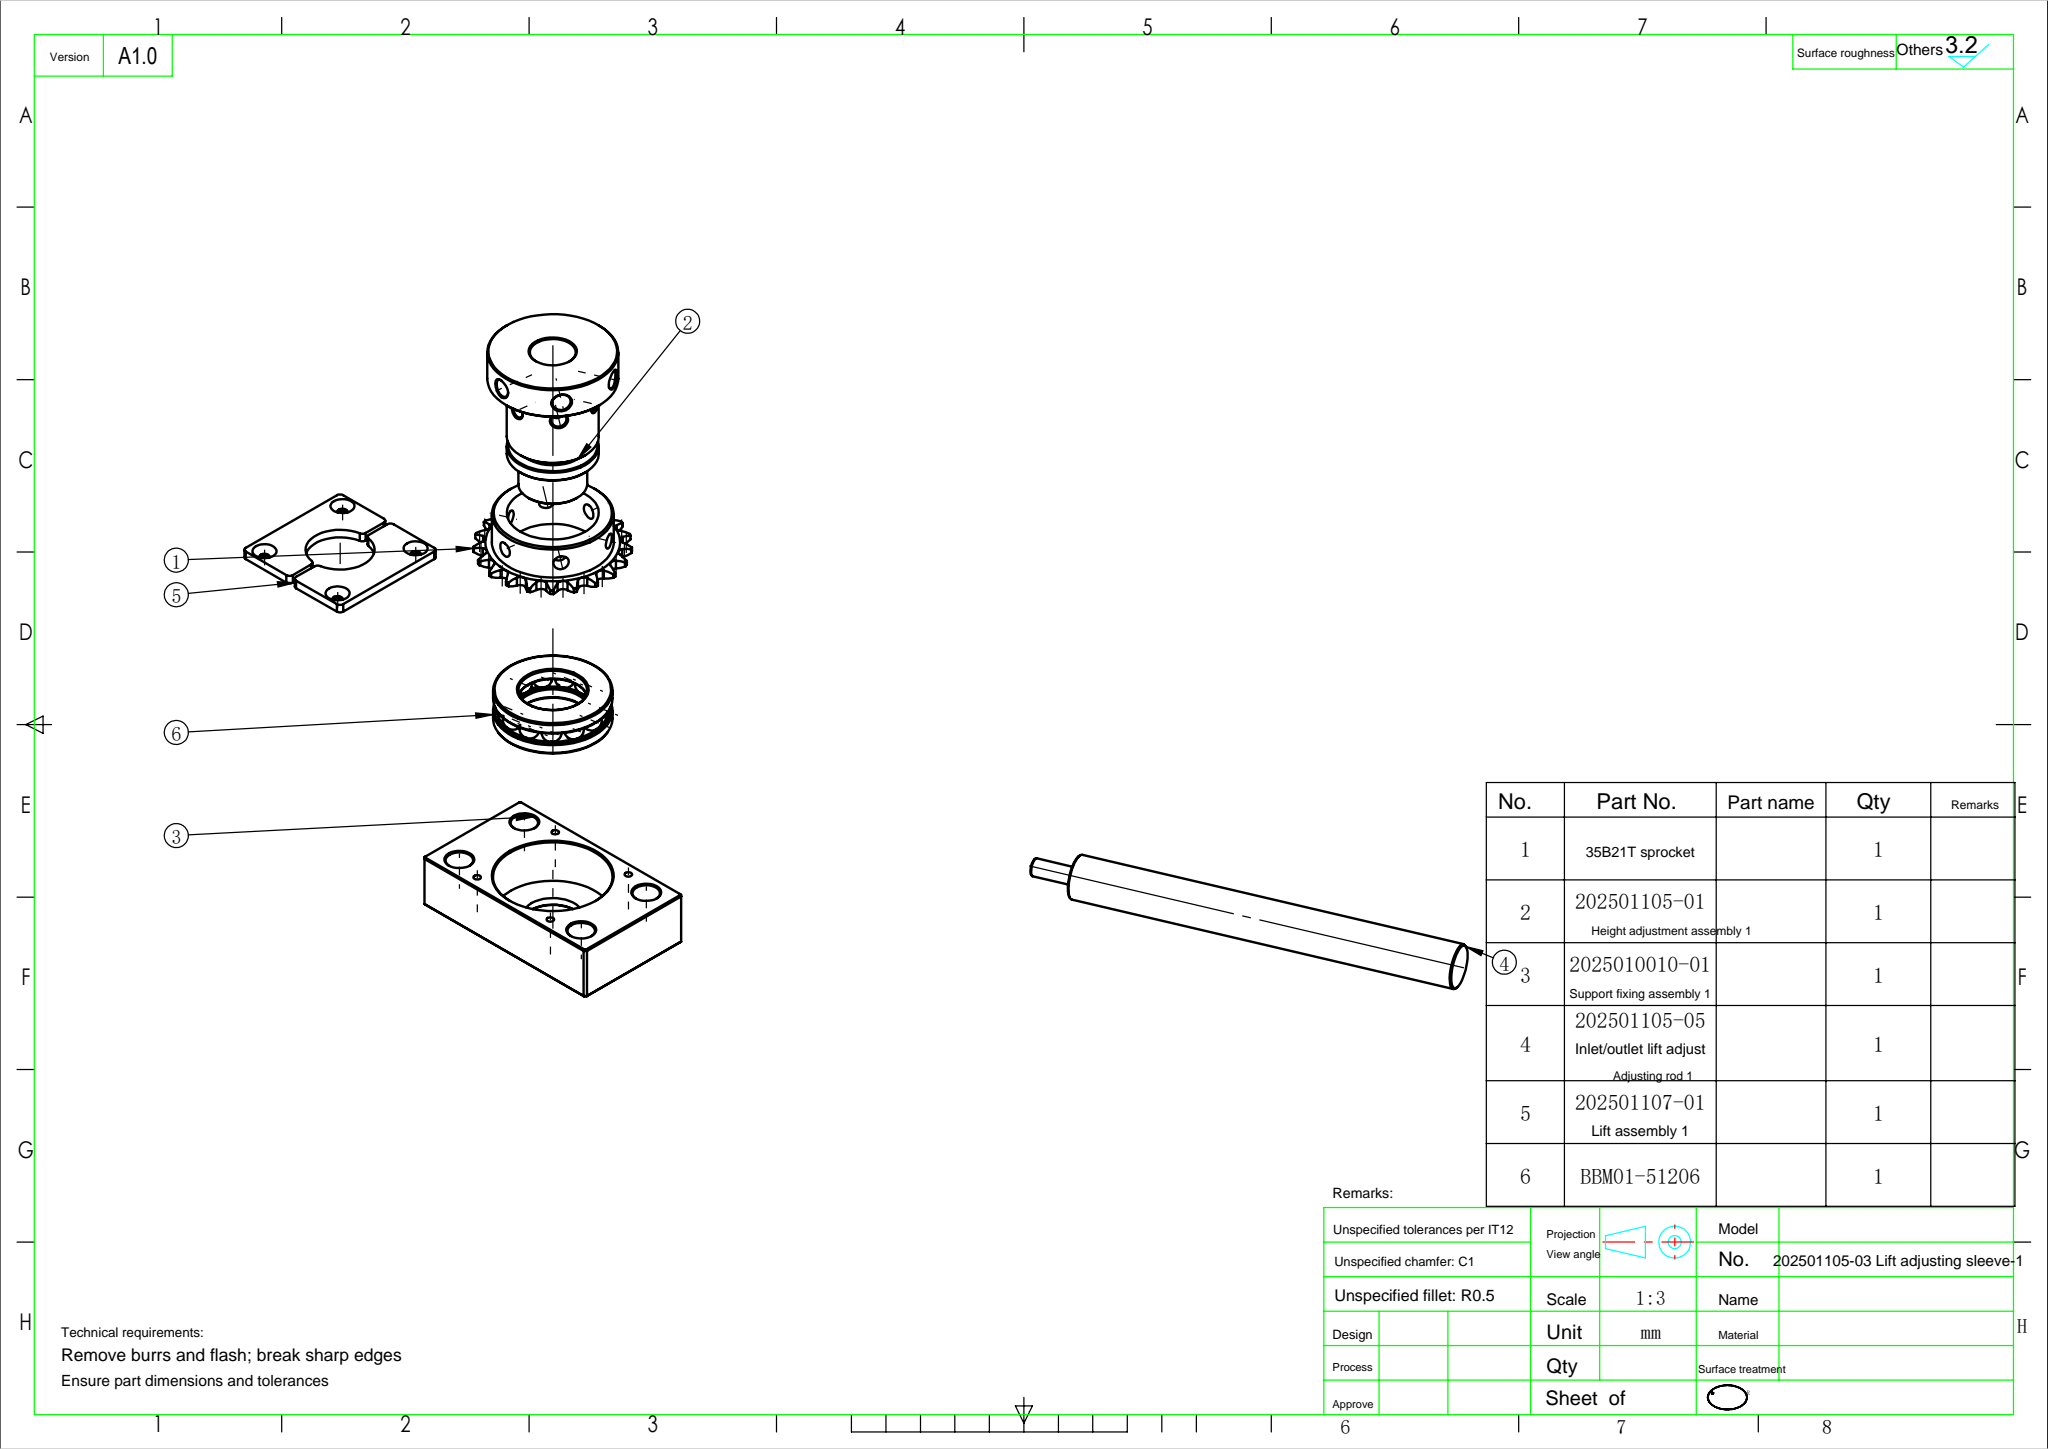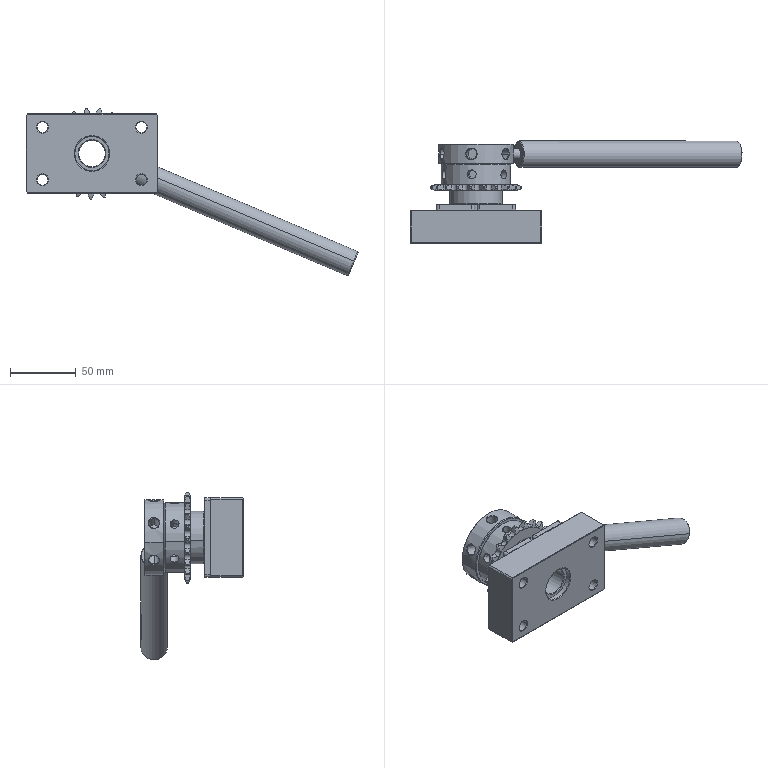Part | SolidWorks | 7 solids | 435 faces | box 251.752 x 77.5 x 127.178 mm | volume 270246 mm3 | cylinder 164 | plane 121 | spline 98 | cone 52 | commonest cylinder face diameters 5.2 x28 6.8 x24 69 x21 4 x12 8.1 x12 30 x9